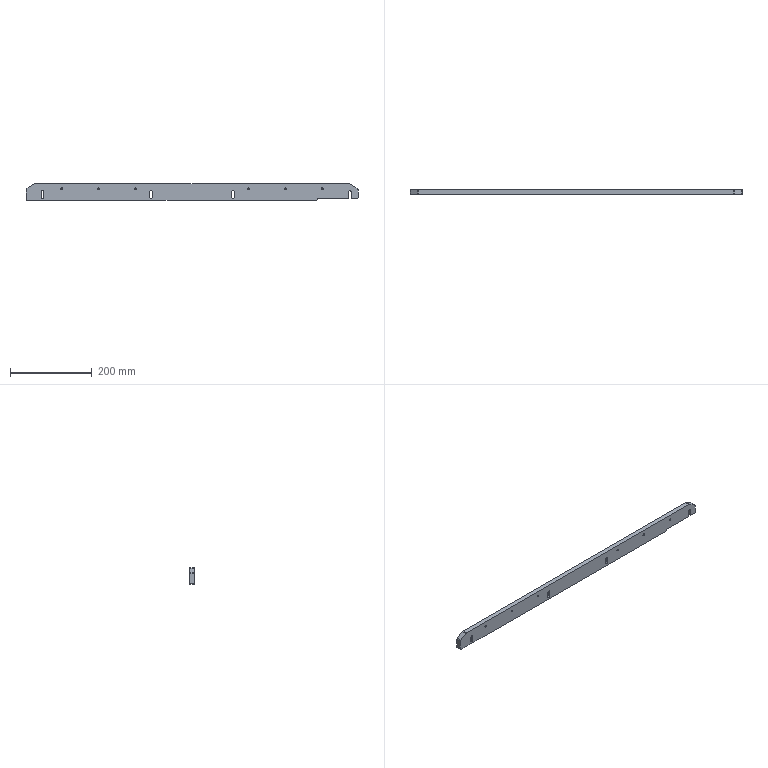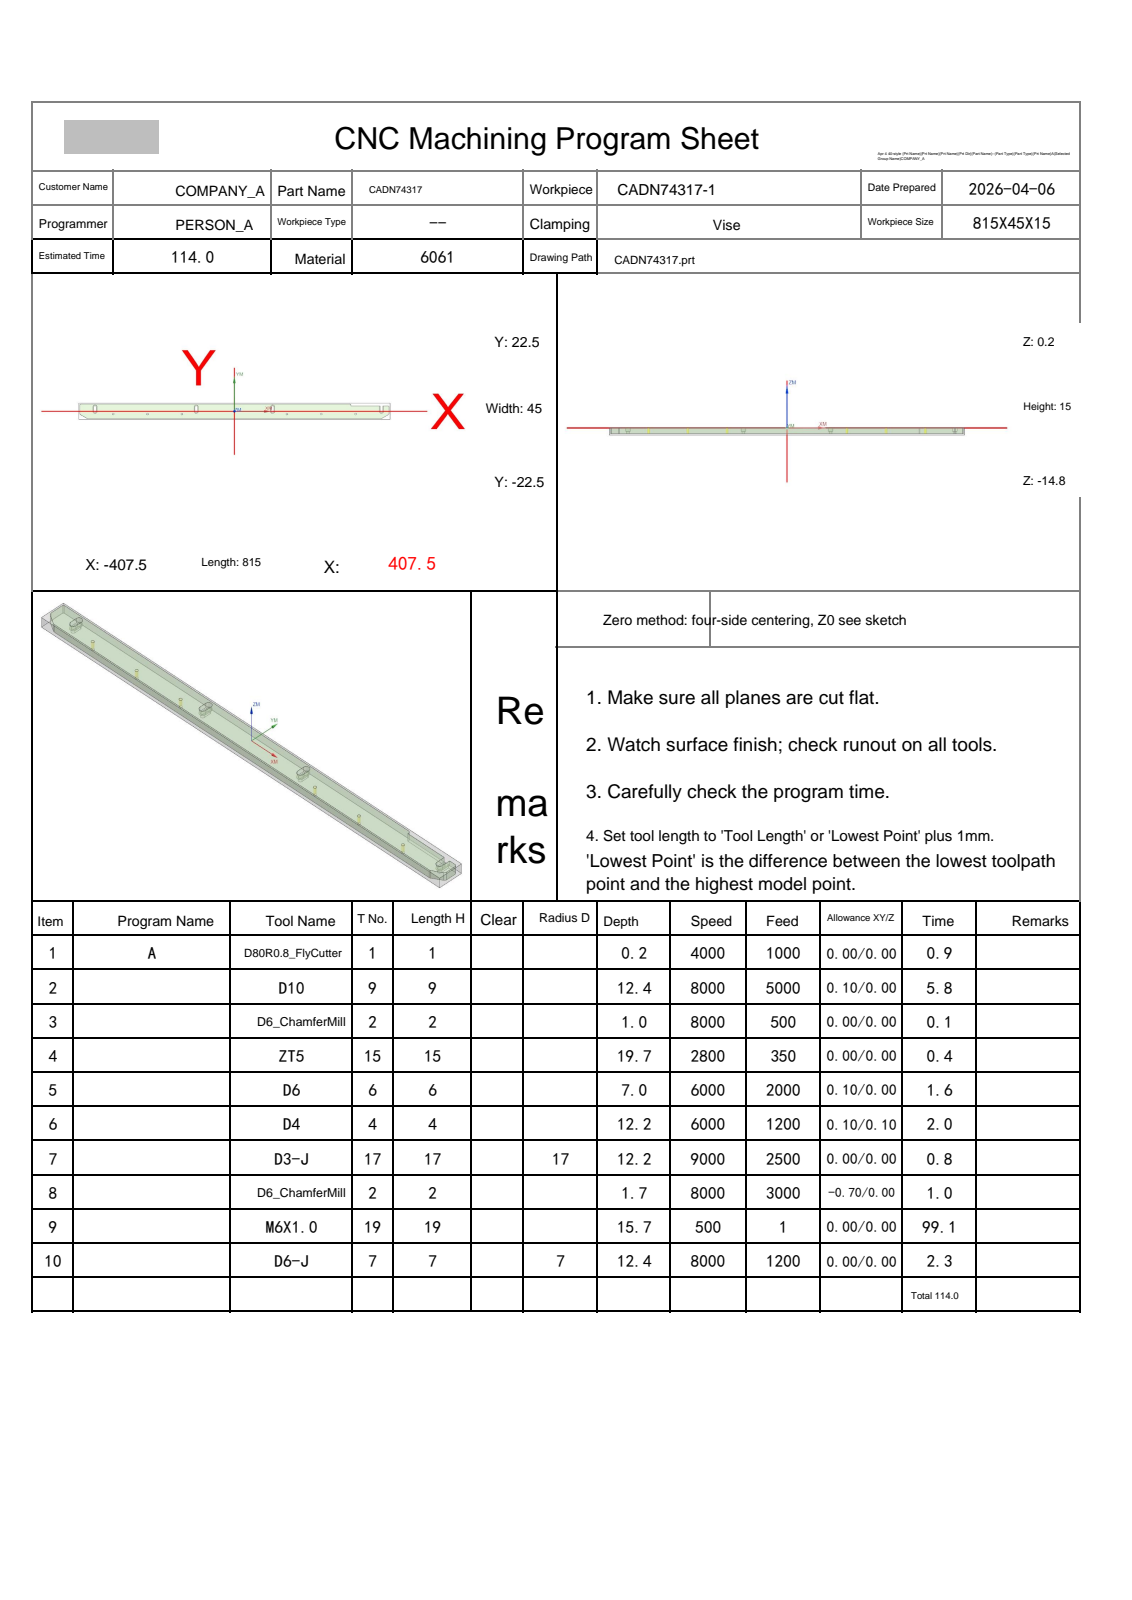NC program | NX | posted by the shop | part box 810 x 12 x 40 mm
Lines 1439 to 3610 of 3610, first 1654 of 2172 lines:
N7 T17 M06
(D3-J  D=3. R=0. H=17 ce=0.00 di=0.00)
G00 G90 G54 X-366.55 Y6.2 M03 S6000
G43 H17 Z20.
M08
Z-8.9
G01 Z-9.4 F800.
G41 D17
X-366.6
G03 X-366.8 Y6. I0.0 J-.2
G01 Y0.0
G03 X-365. Y-1.8 I1.8 J0.0
X-363.2 Y0.0 I0.0 J1.8
G01 Y12.
G03 X-365. Y13.8 I-1.8 J0.0
X-366.8 Y12. I0.0 J-1.8
G01 Y6.
Y5.5
G03 X-366.6 Y5.3 I.2 J0.0
G01 G40 X-366.55
Z-8.9
G00 Z-5.8
Y6.2
Z-11.5
G01 Z-12.
G41 D17
X-366.6
G03 X-366.8 Y6. I0.0 J-.2
G01 Y0.0
G03 X-365. Y-1.8 I1.8 J0.0
X-363.2 Y0.0 I0.0 J1.8
G01 Y12.
G03 X-365. Y13.8 I-1.8 J0.0
X-366.8 Y12. I0.0 J-1.8
G01 Y6.
Y5.5
G03 X-366.6 Y5.3 I.2 J0.0
G01 G40 X-366.55
Z-11.5
G00 Z20.
X-101.55 Y6.2
Z-8.9
G01 Z-9.4
G41 D17
X-101.6
G03 X-101.8 Y6. I0.0 J-.2
G01 Y0.0
G03 X-100. Y-1.8 I1.8 J0.0
X-98.2 Y0.0 I0.0 J1.8
G01 Y12.
G03 X-100. Y13.8 I-1.8 J0.0
X-101.8 Y12. I0.0 J-1.8
G01 Y6.
Y5.5
G03 X-101.6 Y5.3 I.2 J0.0
G01 G40 X-101.55
Z-8.9
G00 Z-5.8
Y6.2
Z-11.5
G01 Z-12.
G41 D17
X-101.6
G03 X-101.8 Y6. I0.0 J-.2
G01 Y0.0
G03 X-100. Y-1.8 I1.8 J0.0
X-98.2 Y0.0 I0.0 J1.8
G01 Y12.
G03 X-100. Y13.8 I-1.8 J0.0
X-101.8 Y12. I0.0 J-1.8
G01 Y6.
Y5.5
G03 X-101.6 Y5.3 I.2 J0.0
G01 G40 X-101.55
Z-11.5
G00 Z20.
X98.45 Y6.2
Z-8.9
G01 Z-9.4
G41 D17
X98.4
G03 X98.2 Y6. I0.0 J-.2
G01 Y0.0
G03 X100. Y-1.8 I1.8 J0.0
X101.8 Y0.0 I0.0 J1.8
G01 Y12.
G03 X100. Y13.8 I-1.8 J0.0
X98.2 Y12. I0.0 J-1.8
G01 Y6.
Y5.5
G03 X98.4 Y5.3 I.2 J0.0
G01 G40 X98.45
Z-8.9
G00 Z-5.8
Y6.2
Z-11.5
G01 Z-12.
G41 D17
X98.4
G03 X98.2 Y6. I0.0 J-.2
G01 Y0.0
G03 X100. Y-1.8 I1.8 J0.0
X101.8 Y0.0 I0.0 J1.8
G01 Y12.
G03 X100. Y13.8 I-1.8 J0.0
X98.2 Y12. I0.0 J-1.8
G01 Y6.
Y5.5
G03 X98.4 Y5.3 I.2 J0.0
G01 G40 X98.45
Z-11.5
G00 Z20.
G00 G90 X306.441 Y19.378 M03 S9000
Z20.
Z.151
G01 X306.438 Y19.374 Z.087 F2000.
X306.427 Y19.364 Z.029
X306.41 Y19.347 Z-.024
X306.389 Y19.324 Z-.071
X306.365 Y19.297 Z-.113
X306.338 Y19.266 Z-.149
X306.311 Y19.23 Z-.181
X306.284 Y19.192 Z-.209
X306.259 Y19.152 Z-.232
X306.236 Y19.109 Z-.251
X306.218 Y19.066 Z-.267
X306.205 Y19.023 Z-.279
X306.198 Y18.98 Z-.288
X306.2 Y18.937 Z-.294
X306.21 Y18.897 Z-.298
X306.23 Y18.859 Z-.299
G02 X306.5 Y18. I-1.23 J-.859 F2500.
G01 Y16.5
X309.708
X309.736 Y16.513 Z-.3
X309.741 Y16.549 Z-.302
X309.723 Y16.606 Z-.306
X309.685 Y16.681 Z-.312
X309.628 Y16.772 Z-.319
X309.555 Y16.876 Z-.327
X309.467 Y16.99 Z-.336
X309.307 Y17.178 Z-.352
X309.191 Y17.305 Z-.363
X309.004 Y17.495 Z-.38
X308.702 Y17.767 Z-.406
X308.379 Y18.02 Z-.434
X308.039 Y18.249 Z-.462
X307.689 Y18.451 Z-.49
X307.333 Y18.621 Z-.517
X307.155 Y18.693 Z-.529
X306.982 Y18.756 Z-.542
X306.816 Y18.808 Z-.553
X306.663 Y18.85 Z-.564
X306.526 Y18.882 Z-.573
X306.41 Y18.902 Z-.582
X306.318 Y18.91 Z-.588
X306.255 Y18.906 Z-.593
X306.224 Y18.889 Z-.596
X306.23 Y18.859 Z-.598
G02 X306.5 Y18. I-1.23 J-.859
G01 Y16.5
X309.708
X309.736 Y16.513
X309.741 Y16.549 Z-.601
X309.723 Y16.606 Z-.605
X309.685 Y16.681 Z-.611
X309.628 Y16.772 Z-.618
X309.555 Y16.876 Z-.626
X309.467 Y16.99 Z-.635
X309.307 Y17.178 Z-.65
X309.191 Y17.305 Z-.661
X309.004 Y17.495 Z-.678
X308.702 Y17.767 Z-.705
X308.379 Y18.02 Z-.733
X308.039 Y18.249 Z-.761
X307.689 Y18.451 Z-.789
X307.333 Y18.621 Z-.815
X307.155 Y18.693 Z-.828
X306.982 Y18.756 Z-.84
X306.816 Y18.808 Z-.852
X306.663 Y18.85 Z-.863
X306.526 Y18.882 Z-.872
X306.41 Y18.902 Z-.88
X306.318 Y18.91 Z-.887
X306.255 Y18.906 Z-.892
X306.224 Y18.889 Z-.895
X306.23 Y18.859 Z-.896
G02 X306.5 Y18. I-1.23 J-.859
G01 Y16.5
X309.708
X309.736 Y16.513 Z-.897
X309.741 Y16.549 Z-.9
X309.723 Y16.606 Z-.904
X309.685 Y16.681 Z-.91
X309.628 Y16.772 Z-.916
X309.555 Y16.876 Z-.925
X309.467 Y16.99 Z-.934
X309.307 Y17.178 Z-.949
X309.191 Y17.305 Z-.96
X309.004 Y17.495 Z-.977
X308.702 Y17.767 Z-1.004
X308.379 Y18.02 Z-1.032
X308.039 Y18.249 Z-1.06
X307.689 Y18.451 Z-1.087
X307.333 Y18.621 Z-1.114
X307.155 Y18.693 Z-1.127
X306.982 Y18.756 Z-1.139
X306.816 Y18.808 Z-1.151
X306.663 Y18.85 Z-1.161
X306.526 Y18.882 Z-1.171
X306.41 Y18.902 Z-1.179
X306.318 Y18.91 Z-1.186
X306.255 Y18.906 Z-1.191
X306.224 Y18.889 Z-1.194
X306.23 Y18.859 Z-1.195
G02 X306.5 Y18. I-1.23 J-.859
G01 Y16.5
X309.708
X309.736 Y16.513 Z-1.196
X309.741 Y16.549 Z-1.199
X309.723 Y16.606 Z-1.203
X309.685 Y16.681 Z-1.208
X309.628 Y16.772 Z-1.215
X309.555 Y16.876 Z-1.223
X309.467 Y16.99 Z-1.232
X309.307 Y17.178 Z-1.248
X309.191 Y17.305 Z-1.259
X309.004 Y17.495 Z-1.276
X308.702 Y17.767 Z-1.303
X308.379 Y18.02 Z-1.33
X308.039 Y18.249 Z-1.358
X307.689 Y18.451 Z-1.386
X307.333 Y18.621 Z-1.413
X307.155 Y18.693 Z-1.426
X306.982 Y18.756 Z-1.438
X306.816 Y18.808 Z-1.45
X306.663 Y18.85 Z-1.46
X306.526 Y18.882 Z-1.47
X306.41 Y18.902 Z-1.478
X306.318 Y18.91 Z-1.485
X306.255 Y18.906 Z-1.49
X306.224 Y18.889 Z-1.493
X306.23 Y18.859 Z-1.494
G02 X306.5 Y18. I-1.23 J-.859
G01 Y16.5
X309.708
X309.736 Y16.513 Z-1.495
X309.741 Y16.549 Z-1.497
X309.723 Y16.606 Z-1.501
X309.685 Y16.681 Z-1.507
X309.628 Y16.772 Z-1.514
X309.555 Y16.876 Z-1.522
X309.467 Y16.99 Z-1.531
X309.307 Y17.178 Z-1.547
X309.191 Y17.305 Z-1.558
X309.004 Y17.495 Z-1.575
X308.702 Y17.767 Z-1.601
X308.379 Y18.02 Z-1.629
X308.039 Y18.249 Z-1.657
X307.689 Y18.451 Z-1.685
X307.333 Y18.621 Z-1.712
X307.155 Y18.693 Z-1.724
X306.982 Y18.756 Z-1.737
X306.816 Y18.808 Z-1.748
X306.663 Y18.85 Z-1.759
X306.526 Y18.882 Z-1.768
X306.41 Y18.902 Z-1.777
X306.318 Y18.91 Z-1.783
X306.255 Y18.906 Z-1.788
X306.224 Y18.889 Z-1.791
X306.23 Y18.859 Z-1.793
G02 X306.5 Y18. I-1.23 J-.859
G01 Y16.5
X309.708
X309.736 Y16.513
X309.741 Y16.549 Z-1.796
X309.723 Y16.606 Z-1.8
X309.685 Y16.681 Z-1.806
X309.628 Y16.772 Z-1.813
X309.555 Y16.876 Z-1.821
X309.467 Y16.99 Z-1.83
X309.307 Y17.178 Z-1.845
X309.191 Y17.305 Z-1.856
X309.004 Y17.495 Z-1.873
X308.702 Y17.767 Z-1.9
X308.379 Y18.02 Z-1.928
X308.039 Y18.249 Z-1.956
X307.689 Y18.451 Z-1.984
X307.333 Y18.621 Z-2.01
X307.155 Y18.693 Z-2.023
X306.982 Y18.756 Z-2.035
X306.816 Y18.808 Z-2.047
X306.663 Y18.85 Z-2.058
X306.526 Y18.882 Z-2.067
X306.41 Y18.902 Z-2.075
X306.318 Y18.91 Z-2.082
X306.255 Y18.906 Z-2.087
X306.224 Y18.889 Z-2.09
X306.23 Y18.859 Z-2.091
G02 X306.5 Y18. I-1.23 J-.859
G01 Y16.5
X309.708
X309.736 Y16.513 Z-2.092
X309.741 Y16.549 Z-2.095
X309.723 Y16.606 Z-2.099
X309.685 Y16.681 Z-2.105
X309.628 Y16.772 Z-2.111
X309.555 Y16.876 Z-2.12
X309.467 Y16.99 Z-2.129
X309.307 Y17.178 Z-2.144
X309.191 Y17.305 Z-2.155
X309.004 Y17.495 Z-2.172
X308.702 Y17.767 Z-2.199
X308.379 Y18.02 Z-2.227
X308.039 Y18.249 Z-2.255
X307.689 Y18.451 Z-2.282
X307.333 Y18.621 Z-2.309
X307.155 Y18.693 Z-2.322
X306.982 Y18.756 Z-2.334
X306.816 Y18.808 Z-2.346
X306.663 Y18.85 Z-2.356
X306.526 Y18.882 Z-2.366
X306.41 Y18.902 Z-2.374
X306.318 Y18.91 Z-2.381
X306.255 Y18.906 Z-2.386
X306.224 Y18.889 Z-2.389
X306.23 Y18.859 Z-2.39
G02 X306.5 Y18. I-1.23 J-.859
G01 Y16.5
X309.708
X309.736 Y16.513 Z-2.391
X309.741 Y16.549 Z-2.394
X309.723 Y16.606 Z-2.398
X309.685 Y16.681 Z-2.403
X309.628 Y16.772 Z-2.41
X309.555 Y16.876 Z-2.418
X309.467 Y16.99 Z-2.427
X309.307 Y17.178 Z-2.443
X309.191 Y17.305 Z-2.454
X309.004 Y17.495 Z-2.471
X308.702 Y17.767 Z-2.498
X308.379 Y18.02 Z-2.525
X308.039 Y18.249 Z-2.553
X307.689 Y18.451 Z-2.581
X307.333 Y18.621 Z-2.608
X307.155 Y18.693 Z-2.621
X306.982 Y18.756 Z-2.633
X306.816 Y18.808 Z-2.645
X306.663 Y18.85 Z-2.655
X306.526 Y18.882 Z-2.665
X306.41 Y18.902 Z-2.673
X306.318 Y18.91 Z-2.68
X306.255 Y18.906 Z-2.685
X306.224 Y18.889 Z-2.688
X306.23 Y18.859 Z-2.689
G02 X306.5 Y18. I-1.23 J-.859
G01 Y16.5
X309.708
X309.736 Y16.513 Z-2.69
X309.741 Y16.549 Z-2.692
X309.723 Y16.606 Z-2.696
X309.685 Y16.681 Z-2.702
X309.628 Y16.772 Z-2.709
X309.555 Y16.876 Z-2.717
X309.467 Y16.99 Z-2.726
X309.307 Y17.178 Z-2.742
X309.191 Y17.305 Z-2.753
X309.004 Y17.495 Z-2.77
X308.702 Y17.767 Z-2.796
X308.379 Y18.02 Z-2.824
X308.039 Y18.249 Z-2.852
X307.689 Y18.451 Z-2.88
X307.333 Y18.621 Z-2.907
X307.155 Y18.693 Z-2.919
X306.982 Y18.756 Z-2.932
X306.816 Y18.808 Z-2.943
X306.663 Y18.85 Z-2.954
X306.526 Y18.882 Z-2.963
X306.41 Y18.902 Z-2.972
X306.318 Y18.91 Z-2.978
X306.255 Y18.906 Z-2.983
X306.224 Y18.889 Z-2.986
X306.23 Y18.859 Z-2.988
G02 X306.5 Y18. I-1.23 J-.859
G01 Y16.5
X309.708
X309.736 Y16.513
X309.741 Y16.549 Z-2.991
X309.723 Y16.606 Z-2.995
X309.685 Y16.681 Z-3.001
X309.628 Y16.772 Z-3.008
X309.555 Y16.876 Z-3.016
X309.467 Y16.99 Z-3.025
X309.307 Y17.178 Z-3.04
X309.191 Y17.305 Z-3.051
X309.004 Y17.495 Z-3.068
X308.702 Y17.767 Z-3.095
X308.379 Y18.02 Z-3.123
X308.039 Y18.249 Z-3.151
X307.689 Y18.451 Z-3.179
X307.333 Y18.621 Z-3.205
X307.155 Y18.693 Z-3.218
X306.982 Y18.756 Z-3.23
X306.816 Y18.808 Z-3.242
X306.663 Y18.85 Z-3.253
X306.526 Y18.882 Z-3.262
X306.41 Y18.902 Z-3.27
X306.318 Y18.91 Z-3.277
X306.255 Y18.906 Z-3.282
X306.224 Y18.889 Z-3.285
X306.23 Y18.859 Z-3.286
G02 X306.5 Y18. I-1.23 J-.859
G01 Y16.5
X309.708
X309.736 Y16.513 Z-3.287
X309.741 Y16.549 Z-3.29
X309.723 Y16.606 Z-3.294
X309.685 Y16.681 Z-3.3
X309.628 Y16.772 Z-3.306
X309.555 Y16.876 Z-3.315
X309.467 Y16.99 Z-3.324
X309.307 Y17.178 Z-3.339
X309.191 Y17.305 Z-3.35
X309.004 Y17.495 Z-3.367
X308.702 Y17.767 Z-3.394
X308.379 Y18.02 Z-3.422
X308.039 Y18.249 Z-3.45
X307.689 Y18.451 Z-3.477
X307.333 Y18.621 Z-3.504
X307.155 Y18.693 Z-3.517
X306.982 Y18.756 Z-3.529
X306.816 Y18.808 Z-3.541
X306.663 Y18.85 Z-3.551
X306.526 Y18.882 Z-3.561
X306.41 Y18.902 Z-3.569
X306.318 Y18.91 Z-3.576
X306.255 Y18.906 Z-3.581
X306.224 Y18.889 Z-3.584
X306.23 Y18.859 Z-3.585
G02 X306.5 Y18. I-1.23 J-.859
G01 Y16.5
X309.708
X309.736 Y16.513 Z-3.586
X309.741 Y16.549 Z-3.589
X309.723 Y16.606 Z-3.593
X309.685 Y16.681 Z-3.598
X309.628 Y16.772 Z-3.605
X309.555 Y16.876 Z-3.613
X309.467 Y16.99 Z-3.622
X309.307 Y17.178 Z-3.638
X309.191 Y17.305 Z-3.649
X309.004 Y17.495 Z-3.666
X308.702 Y17.767 Z-3.693
X308.379 Y18.02 Z-3.72
X308.039 Y18.249 Z-3.748
X307.689 Y18.451 Z-3.776
X307.333 Y18.621 Z-3.803
X307.155 Y18.693 Z-3.816
X306.982 Y18.756 Z-3.828
X306.816 Y18.808 Z-3.84
X306.663 Y18.85 Z-3.85
X306.526 Y18.882 Z-3.86
X306.41 Y18.902 Z-3.868
X306.318 Y18.91 Z-3.875
X306.255 Y18.906 Z-3.88
X306.224 Y18.889 Z-3.883
X306.23 Y18.859 Z-3.884
G02 X306.5 Y18. I-1.23 J-.859
G01 Y16.5
X309.708
X309.736 Y16.513 Z-3.885
X309.741 Y16.549 Z-3.887
X309.723 Y16.606 Z-3.891
X309.685 Y16.681 Z-3.897
X309.628 Y16.772 Z-3.904
X309.555 Y16.876 Z-3.912
X309.467 Y16.99 Z-3.921
X309.307 Y17.178 Z-3.937
X309.191 Y17.305 Z-3.948
X309.004 Y17.495 Z-3.965
X308.702 Y17.767 Z-3.991
X308.379 Y18.02 Z-4.019
X308.039 Y18.249 Z-4.047
X307.689 Y18.451 Z-4.075
X307.333 Y18.621 Z-4.102
X307.155 Y18.693 Z-4.114
X306.982 Y18.756 Z-4.127
X306.816 Y18.808 Z-4.138
X306.663 Y18.85 Z-4.149
X306.526 Y18.882 Z-4.158
X306.41 Y18.902 Z-4.167
X306.318 Y18.91 Z-4.173
X306.255 Y18.906 Z-4.178
X306.224 Y18.889 Z-4.181
X306.23 Y18.859 Z-4.183
G02 X306.5 Y18. I-1.23 J-.859
G01 Y16.5
X309.708
X309.736 Y16.513
X309.741 Y16.549 Z-4.186
X309.723 Y16.606 Z-4.19
X309.685 Y16.681 Z-4.196
X309.628 Y16.772 Z-4.203
X309.555 Y16.876 Z-4.211
X309.467 Y16.99 Z-4.22
X309.307 Y17.178 Z-4.235
X309.191 Y17.305 Z-4.246
X309.004 Y17.495 Z-4.263
X308.702 Y17.767 Z-4.29
X308.379 Y18.02 Z-4.318
X308.039 Y18.249 Z-4.346
X307.689 Y18.451 Z-4.374
X307.333 Y18.621 Z-4.4
X307.155 Y18.693 Z-4.413
X306.982 Y18.756 Z-4.425
X306.816 Y18.808 Z-4.437
X306.663 Y18.85 Z-4.448
X306.526 Y18.882 Z-4.457
X306.41 Y18.902 Z-4.465
X306.318 Y18.91 Z-4.472
X306.255 Y18.906 Z-4.477
X306.224 Y18.889 Z-4.48
X306.23 Y18.859 Z-4.481
G02 X306.5 Y18. I-1.23 J-.859
G01 Y16.5
X309.708
X309.736 Y16.513 Z-4.482
X309.741 Y16.549 Z-4.485
X309.723 Y16.606 Z-4.489
X309.685 Y16.681 Z-4.495
X309.628 Y16.772 Z-4.501
X309.555 Y16.876 Z-4.51
X309.467 Y16.99 Z-4.519
X309.307 Y17.178 Z-4.534
X309.191 Y17.305 Z-4.545
X309.004 Y17.495 Z-4.562
X308.702 Y17.767 Z-4.589
X308.379 Y18.02 Z-4.617
X308.039 Y18.249 Z-4.645
X307.689 Y18.451 Z-4.672
X307.333 Y18.621 Z-4.699
X307.155 Y18.693 Z-4.712
X306.982 Y18.756 Z-4.724
X306.816 Y18.808 Z-4.736
X306.663 Y18.85 Z-4.746
X306.526 Y18.882 Z-4.756
X306.41 Y18.902 Z-4.764
X306.318 Y18.91 Z-4.771
X306.255 Y18.906 Z-4.776
X306.224 Y18.889 Z-4.779
X306.23 Y18.859 Z-4.78
G02 X306.5 Y18. I-1.23 J-.859
G01 Y16.5
X309.708
X309.736 Y16.513 Z-4.781
X309.741 Y16.549 Z-4.784
X309.723 Y16.606 Z-4.788
X309.685 Y16.681 Z-4.793
X309.628 Y16.772 Z-4.8
X309.555 Y16.876 Z-4.808
X309.467 Y16.99 Z-4.817
X309.307 Y17.178 Z-4.833
X309.191 Y17.305 Z-4.844
X309.004 Y17.495 Z-4.861
X308.702 Y17.767 Z-4.888
X308.379 Y18.02 Z-4.915
X308.039 Y18.249 Z-4.943
X307.689 Y18.451 Z-4.971
X307.333 Y18.621 Z-4.998
X307.155 Y18.693 Z-5.011
X306.982 Y18.756 Z-5.023
X306.816 Y18.808 Z-5.035
X306.663 Y18.85 Z-5.045
X306.526 Y18.882 Z-5.055
X306.41 Y18.902 Z-5.063
X306.318 Y18.91 Z-5.07
X306.255 Y18.906 Z-5.075
X306.224 Y18.889 Z-5.078
X306.23 Y18.859 Z-5.079
G02 X306.5 Y18. I-1.23 J-.859
G01 Y16.5
X309.708
X309.736 Y16.513 Z-5.08
X309.741 Y16.549 Z-5.082
X309.723 Y16.606 Z-5.086
X309.685 Y16.681 Z-5.092
X309.628 Y16.772 Z-5.099
X309.555 Y16.876 Z-5.107
X309.467 Y16.99 Z-5.116
X309.307 Y17.178 Z-5.132
X309.191 Y17.305 Z-5.143
X309.004 Y17.495 Z-5.16
X308.702 Y17.767 Z-5.186
X308.379 Y18.02 Z-5.214
X308.039 Y18.249 Z-5.242
X307.689 Y18.451 Z-5.27
X307.333 Y18.621 Z-5.297
X307.155 Y18.693 Z-5.309
X306.982 Y18.756 Z-5.322
X306.816 Y18.808 Z-5.333
X306.663 Y18.85 Z-5.344
X306.526 Y18.882 Z-5.353
X306.41 Y18.902 Z-5.362
X306.318 Y18.91 Z-5.368
X306.255 Y18.906 Z-5.373
X306.224 Y18.889 Z-5.376
X306.23 Y18.859 Z-5.378
G02 X306.5 Y18. I-1.23 J-.859
G01 Y16.5
X309.708
X309.736 Y16.513
X309.741 Y16.549 Z-5.381
X309.723 Y16.606 Z-5.385
X309.685 Y16.681 Z-5.391
X309.628 Y16.772 Z-5.398
X309.555 Y16.876 Z-5.406
X309.467 Y16.99 Z-5.415
X309.307 Y17.178 Z-5.43
X309.191 Y17.305 Z-5.441
X309.004 Y17.495 Z-5.458
X308.702 Y17.767 Z-5.485
X308.379 Y18.02 Z-5.513
X308.039 Y18.249 Z-5.541
X307.689 Y18.451 Z-5.569
X307.333 Y18.621 Z-5.595
X307.155 Y18.693 Z-5.608
X306.982 Y18.756 Z-5.62
X306.816 Y18.808 Z-5.632
X306.663 Y18.85 Z-5.643
X306.526 Y18.882 Z-5.652
X306.41 Y18.902 Z-5.66
X306.318 Y18.91 Z-5.667
X306.255 Y18.906 Z-5.672
X306.224 Y18.889 Z-5.675
X306.23 Y18.859 Z-5.676
G02 X306.5 Y18. I-1.23 J-.859
G01 Y16.5
X309.708
X309.736 Y16.513 Z-5.677
X309.741 Y16.549 Z-5.68
X309.723 Y16.606 Z-5.684
X309.685 Y16.681 Z-5.69
X309.628 Y16.772 Z-5.696
X309.555 Y16.876 Z-5.705
X309.467 Y16.99 Z-5.714
X309.307 Y17.178 Z-5.729
X309.191 Y17.305 Z-5.74
X309.004 Y17.495 Z-5.757
X308.702 Y17.767 Z-5.784
X308.379 Y18.02 Z-5.812
X308.039 Y18.249 Z-5.84
X307.689 Y18.451 Z-5.867
X307.333 Y18.621 Z-5.894
X307.155 Y18.693 Z-5.907
X306.982 Y18.756 Z-5.919
X306.816 Y18.808 Z-5.931
X306.663 Y18.85 Z-5.941
X306.526 Y18.882 Z-5.951
X306.41 Y18.902 Z-5.959
X306.318 Y18.91 Z-5.966
X306.255 Y18.906 Z-5.971
X306.224 Y18.889 Z-5.974
X306.23 Y18.859 Z-5.975
G02 X306.5 Y18. I-1.23 J-.859
G01 Y16.5
X309.708
X309.736 Y16.513 Z-5.976
X309.741 Y16.549 Z-5.979
X309.723 Y16.606 Z-5.983
X309.685 Y16.681 Z-5.988
X309.628 Y16.772 Z-5.995
X309.555 Y16.876 Z-6.003
X309.467 Y16.99 Z-6.012
X309.307 Y17.178 Z-6.028
X309.191 Y17.305 Z-6.039
X309.004 Y17.495 Z-6.056
X308.702 Y17.767 Z-6.083
X308.379 Y18.02 Z-6.11
X308.039 Y18.249 Z-6.138
X307.689 Y18.451 Z-6.166
X307.333 Y18.621 Z-6.193
X307.155 Y18.693 Z-6.206
X306.982 Y18.756 Z-6.218
X306.816 Y18.808 Z-6.23
X306.663 Y18.85 Z-6.24
X306.526 Y18.882 Z-6.25
X306.41 Y18.902 Z-6.258
X306.318 Y18.91 Z-6.265
X306.255 Y18.906 Z-6.27
X306.224 Y18.889 Z-6.273
X306.23 Y18.859 Z-6.274
G02 X306.5 Y18. I-1.23 J-.859
G01 Y16.5
X309.708
X309.736 Y16.513 Z-6.275
X309.741 Y16.549 Z-6.277
X309.723 Y16.606 Z-6.281
X309.685 Y16.681 Z-6.287
X309.628 Y16.772 Z-6.294
X309.555 Y16.876 Z-6.302
X309.467 Y16.99 Z-6.311
X309.307 Y17.178 Z-6.327
X309.191 Y17.305 Z-6.338
X309.004 Y17.495 Z-6.355
X308.702 Y17.767 Z-6.381
X308.379 Y18.02 Z-6.409
X308.039 Y18.249 Z-6.437
X307.689 Y18.451 Z-6.465
X307.333 Y18.621 Z-6.492
X307.155 Y18.693 Z-6.504
X306.982 Y18.756 Z-6.517
X306.816 Y18.808 Z-6.528
X306.663 Y18.85 Z-6.539
X306.526 Y18.882 Z-6.548
X306.41 Y18.902 Z-6.557
X306.318 Y18.91 Z-6.563
X306.255 Y18.906 Z-6.568
X306.224 Y18.889 Z-6.571
X306.23 Y18.859 Z-6.573
G02 X306.5 Y18. I-1.23 J-.859
G01 Y16.5
X309.708
X309.736 Y16.513
X309.741 Y16.549 Z-6.576
X309.723 Y16.606 Z-6.58
X309.685 Y16.681 Z-6.586
X309.628 Y16.772 Z-6.593
X309.555 Y16.876 Z-6.601
X309.467 Y16.99 Z-6.61
X309.307 Y17.178 Z-6.625
X309.191 Y17.305 Z-6.636
X309.004 Y17.495 Z-6.653
X308.702 Y17.767 Z-6.68
X308.379 Y18.02 Z-6.708
X308.039 Y18.249 Z-6.736
X307.689 Y18.451 Z-6.764
X307.333 Y18.621 Z-6.79
X307.155 Y18.693 Z-6.803
X306.982 Y18.756 Z-6.815
X306.816 Y18.808 Z-6.827
X306.663 Y18.85 Z-6.838
X306.526 Y18.882 Z-6.847
X306.41 Y18.902 Z-6.855
X306.318 Y18.91 Z-6.862
X306.255 Y18.906 Z-6.867
X306.224 Y18.889 Z-6.87
X306.23 Y18.859 Z-6.871
G02 X306.5 Y18. I-1.23 J-.859
G01 Y16.5
X309.708
X309.736 Y16.513 Z-6.872
X309.741 Y16.549 Z-6.875
X309.723 Y16.606 Z-6.879
X309.685 Y16.681 Z-6.885
X309.628 Y16.772 Z-6.891
X309.555 Y16.876 Z-6.9
X309.467 Y16.99 Z-6.909
X309.307 Y17.178 Z-6.924
X309.191 Y17.305 Z-6.935
X309.004 Y17.495 Z-6.952
X308.702 Y17.767 Z-6.979
X308.379 Y18.02 Z-7.007
X308.039 Y18.249 Z-7.035
X307.689 Y18.451 Z-7.062
X307.333 Y18.621 Z-7.089
X307.155 Y18.693 Z-7.102
X306.982 Y18.756 Z-7.114
X306.816 Y18.808 Z-7.126
X306.663 Y18.85 Z-7.136
X306.526 Y18.882 Z-7.146
X306.41 Y18.902 Z-7.154
X306.318 Y18.91 Z-7.161
X306.255 Y18.906 Z-7.166
X306.224 Y18.889 Z-7.169
X306.23 Y18.859 Z-7.17
G02 X306.5 Y18. I-1.23 J-.859
G01 Y16.5
X309.708
X309.736 Y16.513 Z-7.171
X309.741 Y16.549 Z-7.174
X309.723 Y16.606 Z-7.178
X309.685 Y16.681 Z-7.183
X309.628 Y16.772 Z-7.19
X309.555 Y16.876 Z-7.198
X309.467 Y16.99 Z-7.207
X309.307 Y17.178 Z-7.223
X309.191 Y17.305 Z-7.234
X309.004 Y17.495 Z-7.251
X308.702 Y17.767 Z-7.278
X308.379 Y18.02 Z-7.305
X308.039 Y18.249 Z-7.333
X307.689 Y18.451 Z-7.361
X307.333 Y18.621 Z-7.388
X307.155 Y18.693 Z-7.401
X306.982 Y18.756 Z-7.413
X306.816 Y18.808 Z-7.425
X306.663 Y18.85 Z-7.435
X306.526 Y18.882 Z-7.445
X306.41 Y18.902 Z-7.453
X306.318 Y18.91 Z-7.46
X306.255 Y18.906 Z-7.465
X306.224 Y18.889 Z-7.468
X306.23 Y18.859 Z-7.469
G02 X306.5 Y18. I-1.23 J-.859
G01 Y16.5
X309.708
X309.736 Y16.513 Z-7.47
X309.741 Y16.549 Z-7.472
X309.723 Y16.606 Z-7.476
X309.685 Y16.681 Z-7.482
X309.628 Y16.772 Z-7.489
X309.555 Y16.876 Z-7.497
X309.467 Y16.99 Z-7.506
X309.307 Y17.178 Z-7.522
X309.191 Y17.305 Z-7.533
X309.004 Y17.495 Z-7.55
X308.702 Y17.767 Z-7.576
X308.379 Y18.02 Z-7.604
X308.039 Y18.249 Z-7.632
X307.689 Y18.451 Z-7.66
X307.333 Y18.621 Z-7.687
X307.155 Y18.693 Z-7.699
X306.982 Y18.756 Z-7.712
X306.816 Y18.808 Z-7.723
X306.663 Y18.85 Z-7.734
X306.526 Y18.882 Z-7.743
X306.41 Y18.902 Z-7.752
X306.318 Y18.91 Z-7.758
X306.255 Y18.906 Z-7.763
X306.224 Y18.889 Z-7.766
X306.23 Y18.859 Z-7.768
G02 X306.5 Y18. I-1.23 J-.859
G01 Y16.5
X309.708
X309.736 Y16.513
X309.741 Y16.549 Z-7.771
X309.723 Y16.606 Z-7.775
X309.685 Y16.681 Z-7.781
X309.628 Y16.772 Z-7.788
X309.555 Y16.876 Z-7.796
X309.467 Y16.99 Z-7.805
X309.307 Y17.178 Z-7.82
X309.191 Y17.305 Z-7.831
X309.004 Y17.495 Z-7.848
X308.702 Y17.767 Z-7.875
X308.379 Y18.02 Z-7.903
X308.039 Y18.249 Z-7.931
X307.689 Y18.451 Z-7.959
X307.333 Y18.621 Z-7.985
X307.155 Y18.693 Z-7.998
X306.982 Y18.756 Z-8.01
X306.816 Y18.808 Z-8.022
X306.663 Y18.85 Z-8.033
X306.526 Y18.882 Z-8.042
X306.41 Y18.902 Z-8.05
X306.318 Y18.91 Z-8.057
X306.255 Y18.906 Z-8.062
X306.224 Y18.889 Z-8.065
X306.23 Y18.859 Z-8.066
G02 X306.5 Y18. I-1.23 J-.859
G01 Y16.5
X309.708
X309.736 Y16.513 Z-8.067
X309.741 Y16.549 Z-8.07
X309.723 Y16.606 Z-8.074
X309.685 Y16.681 Z-8.08
X309.628 Y16.772 Z-8.086
X309.555 Y16.876 Z-8.095
X309.467 Y16.99 Z-8.104
X309.307 Y17.178 Z-8.119
X309.191 Y17.305 Z-8.13
X309.004 Y17.495 Z-8.147
X308.702 Y17.767 Z-8.174
X308.379 Y18.02 Z-8.202
X308.039 Y18.249 Z-8.23
X307.689 Y18.451 Z-8.257
X307.333 Y18.621 Z-8.284
X307.155 Y18.693 Z-8.297
X306.982 Y18.756 Z-8.309
X306.816 Y18.808 Z-8.321
X306.663 Y18.85 Z-8.331
X306.526 Y18.882 Z-8.341
X306.41 Y18.902 Z-8.349
X306.318 Y18.91 Z-8.356
X306.255 Y18.906 Z-8.361
X306.224 Y18.889 Z-8.364
X306.23 Y18.859 Z-8.365
G02 X306.5 Y18. I-1.23 J-.859
G01 Y16.5
X309.708
X309.736 Y16.513 Z-8.366
X309.741 Y16.549 Z-8.369
X309.723 Y16.606 Z-8.373
X309.685 Y16.681 Z-8.378
X309.628 Y16.772 Z-8.385
X309.555 Y16.876 Z-8.393
X309.467 Y16.99 Z-8.402
X309.307 Y17.178 Z-8.418
X309.191 Y17.305 Z-8.429
X309.004 Y17.495 Z-8.446
X308.702 Y17.767 Z-8.473
X308.379 Y18.02 Z-8.5
X308.039 Y18.249 Z-8.528
X307.689 Y18.451 Z-8.556
X307.333 Y18.621 Z-8.583
X307.155 Y18.693 Z-8.596
X306.982 Y18.756 Z-8.608
X306.816 Y18.808 Z-8.62
X306.663 Y18.85 Z-8.63
X306.526 Y18.882 Z-8.64
X306.41 Y18.902 Z-8.648
X306.318 Y18.91 Z-8.655
X306.255 Y18.906 Z-8.66
X306.224 Y18.889 Z-8.663
X306.23 Y18.859 Z-8.664
G02 X306.5 Y18. I-1.23 J-.859
G01 Y16.5
X309.708
X309.736 Y16.513 Z-8.665
X309.741 Y16.549 Z-8.667
X309.723 Y16.606 Z-8.671
X309.685 Y16.681 Z-8.677
X309.628 Y16.772 Z-8.684
X309.555 Y16.876 Z-8.692
X309.467 Y16.99 Z-8.701
X309.307 Y17.178 Z-8.717
X309.191 Y17.305 Z-8.728
X309.004 Y17.495 Z-8.745
X308.702 Y17.767 Z-8.771
X308.379 Y18.02 Z-8.799
X308.039 Y18.249 Z-8.827
X307.689 Y18.451 Z-8.855
X307.333 Y18.621 Z-8.882
X307.155 Y18.693 Z-8.894
X306.982 Y18.756 Z-8.907
X306.816 Y18.808 Z-8.918
X306.663 Y18.85 Z-8.929
X306.526 Y18.882 Z-8.938
X306.41 Y18.902 Z-8.947
X306.318 Y18.91 Z-8.953
X306.255 Y18.906 Z-8.958
X306.224 Y18.889 Z-8.961
X306.23 Y18.859 Z-8.963
G02 X306.5 Y18. I-1.23 J-.859
G01 Y16.5
X309.708
X309.736 Y16.513
X309.741 Y16.549 Z-8.966
X309.723 Y16.606 Z-8.97
X309.685 Y16.681 Z-8.976
X309.628 Y16.772 Z-8.983
X309.555 Y16.876 Z-8.991
X309.467 Y16.99 Z-9.
X309.307 Y17.178 Z-9.015
X309.191 Y17.305 Z-9.026
X309.004 Y17.495 Z-9.043
X308.702 Y17.767 Z-9.07
X308.379 Y18.02 Z-9.098
X308.039 Y18.249 Z-9.126
X307.689 Y18.451 Z-9.154
X307.333 Y18.621 Z-9.18
X307.155 Y18.693 Z-9.193
X306.982 Y18.756 Z-9.205
X306.816 Y18.808 Z-9.217
X306.663 Y18.85 Z-9.228
X306.526 Y18.882 Z-9.237
X306.41 Y18.902 Z-9.245
X306.318 Y18.91 Z-9.252
X306.255 Y18.906 Z-9.257
X306.224 Y18.889 Z-9.26
X306.23 Y18.859 Z-9.261
G02 X306.5 Y18. I-1.23 J-.859
G01 Y16.5
X309.708
X309.736 Y16.513 Z-9.262
X309.741 Y16.549 Z-9.265
X309.723 Y16.606 Z-9.269
X309.685 Y16.681 Z-9.275
X309.628 Y16.772 Z-9.281
X309.555 Y16.876 Z-9.29
X309.467 Y16.99 Z-9.299
X309.307 Y17.178 Z-9.314
X309.191 Y17.305 Z-9.325
X309.004 Y17.495 Z-9.342
X308.702 Y17.767 Z-9.369
X308.379 Y18.02 Z-9.397
X308.039 Y18.249 Z-9.425
X307.689 Y18.451 Z-9.452
X307.333 Y18.621 Z-9.479
X307.155 Y18.693 Z-9.492
X306.982 Y18.756 Z-9.504
X306.816 Y18.808 Z-9.516
X306.663 Y18.85 Z-9.526
X306.526 Y18.882 Z-9.536
X306.41 Y18.902 Z-9.544
X306.318 Y18.91 Z-9.551
X306.255 Y18.906 Z-9.556
X306.224 Y18.889 Z-9.559
X306.23 Y18.859 Z-9.56
G02 X306.5 Y18. I-1.23 J-.859
G01 Y16.5
X309.708
X309.736 Y16.513 Z-9.561
X309.741 Y16.549 Z-9.564
X309.723 Y16.606 Z-9.568
X309.685 Y16.681 Z-9.573
X309.628 Y16.772 Z-9.58
X309.555 Y16.876 Z-9.588
X309.467 Y16.99 Z-9.597
X309.307 Y17.178 Z-9.613
X309.191 Y17.305 Z-9.624
X309.004 Y17.495 Z-9.641
X308.702 Y17.767 Z-9.668
X308.379 Y18.02 Z-9.695
X308.039 Y18.249 Z-9.723
X307.689 Y18.451 Z-9.751
X307.333 Y18.621 Z-9.778
X307.155 Y18.693 Z-9.791
X306.982 Y18.756 Z-9.803
X306.816 Y18.808 Z-9.815
X306.663 Y18.85 Z-9.825
X306.526 Y18.882 Z-9.835
X306.41 Y18.902 Z-9.843
X306.318 Y18.91 Z-9.85
X306.255 Y18.906 Z-9.855
X306.224 Y18.889 Z-9.858
X306.23 Y18.859 Z-9.859
G02 X306.5 Y18. I-1.23 J-.859
G01 Y16.5
X309.708
X309.736 Y16.513 Z-9.86
X309.741 Y16.549 Z-9.862
X309.723 Y16.606 Z-9.866
X309.685 Y16.681 Z-9.872
X309.628 Y16.772 Z-9.879
X309.555 Y16.876 Z-9.887
X309.467 Y16.99 Z-9.896
X309.307 Y17.178 Z-9.912
X309.191 Y17.305 Z-9.923
X309.004 Y17.495 Z-9.94
X308.702 Y17.767 Z-9.966
X308.379 Y18.02 Z-9.994
X308.039 Y18.249 Z-10.022
X307.689 Y18.451 Z-10.05
X307.333 Y18.621 Z-10.077
X307.155 Y18.693 Z-10.089
X306.982 Y18.756 Z-10.102
X306.816 Y18.808 Z-10.113
X306.663 Y18.85 Z-10.124
X306.526 Y18.882 Z-10.133
X306.41 Y18.902 Z-10.142
X306.318 Y18.91 Z-10.148
X306.255 Y18.906 Z-10.153
X306.224 Y18.889 Z-10.156
X306.23 Y18.859 Z-10.158
G02 X306.5 Y18. I-1.23 J-.859
G01 Y16.5
X309.708
X309.736 Y16.513
X309.741 Y16.549 Z-10.161
X309.723 Y16.606 Z-10.165
X309.685 Y16.681 Z-10.171
X309.628 Y16.772 Z-10.178
X309.555 Y16.876 Z-10.186
X309.467 Y16.99 Z-10.195
X309.307 Y17.178 Z-10.21
X309.191 Y17.305 Z-10.221
X309.004 Y17.495 Z-10.238
X308.702 Y17.767 Z-10.265
X308.379 Y18.02 Z-10.293
X308.039 Y18.249 Z-10.321
X307.689 Y18.451 Z-10.349
X307.333 Y18.621 Z-10.375
X307.155 Y18.693 Z-10.388
X306.982 Y18.756 Z-10.4
X306.816 Y18.808 Z-10.412
X306.663 Y18.85 Z-10.423
X306.526 Y18.882 Z-10.432
X306.41 Y18.902 Z-10.44
X306.318 Y18.91 Z-10.447
X306.255 Y18.906 Z-10.452
X306.224 Y18.889 Z-10.455
X306.23 Y18.859 Z-10.456
G02 X306.5 Y18. I-1.23 J-.859
G01 Y16.5
X309.708
X309.736 Y16.513 Z-10.457
X309.741 Y16.549 Z-10.46
X309.723 Y16.606 Z-10.464
X309.685 Y16.681 Z-10.47
X309.628 Y16.772 Z-10.476
X309.555 Y16.876 Z-10.485
X309.467 Y16.99 Z-10.494
X309.307 Y17.178 Z-10.509
X309.191 Y17.305 Z-10.52
X309.004 Y17.495 Z-10.537
X308.702 Y17.767 Z-10.564
X308.379 Y18.02 Z-10.592
X308.039 Y18.249 Z-10.62
X307.689 Y18.451 Z-10.647
X307.333 Y18.621 Z-10.674
X307.155 Y18.693 Z-10.687
X306.982 Y18.756 Z-10.699
X306.816 Y18.808 Z-10.711
X306.663 Y18.85 Z-10.721
X306.526 Y18.882 Z-10.731
X306.41 Y18.902 Z-10.739
X306.318 Y18.91 Z-10.746
X306.255 Y18.906 Z-10.751
X306.224 Y18.889 Z-10.754
X306.23 Y18.859 Z-10.755
G02 X306.5 Y18. I-1.23 J-.859
G01 Y16.5
X309.708
X309.736 Y16.513 Z-10.756
X309.741 Y16.549 Z-10.759
X309.723 Y16.606 Z-10.763
X309.685 Y16.681 Z-10.768
X309.628 Y16.772 Z-10.775
X309.555 Y16.876 Z-10.783
X309.467 Y16.99 Z-10.792
X309.307 Y17.178 Z-10.808
X309.191 Y17.305 Z-10.819
X309.004 Y17.495 Z-10.836
X308.702 Y17.767 Z-10.863
X308.379 Y18.02 Z-10.89
X308.039 Y18.249 Z-10.918
X307.689 Y18.451 Z-10.946
X307.333 Y18.621 Z-10.973
X307.155 Y18.693 Z-10.986
X306.982 Y18.756 Z-10.998
X306.816 Y18.808 Z-11.01
X306.663 Y18.85 Z-11.02
X306.526 Y18.882 Z-11.03
X306.41 Y18.902 Z-11.038
X306.318 Y18.91 Z-11.045
X306.255 Y18.906 Z-11.05
X306.224 Y18.889 Z-11.053
X306.23 Y18.859 Z-11.054
G02 X306.5 Y18. I-1.23 J-.859
G01 Y16.5
X309.708
X309.736 Y16.513 Z-11.055
X309.741 Y16.549 Z-11.057
X309.723 Y16.606 Z-11.061
X309.685 Y16.681 Z-11.067
X309.628 Y16.772 Z-11.074
X309.555 Y16.876 Z-11.082
X309.467 Y16.99 Z-11.091
X309.307 Y17.178 Z-11.107
X309.191 Y17.305 Z-11.118
X309.004 Y17.495 Z-11.135
X308.702 Y17.767 Z-11.161
X308.379 Y18.02 Z-11.189
X308.039 Y18.249 Z-11.217
X307.689 Y18.451 Z-11.245
X307.333 Y18.621 Z-11.272
X307.155 Y18.693 Z-11.284
X306.982 Y18.756 Z-11.297
X306.816 Y18.808 Z-11.308
X306.663 Y18.85 Z-11.319
X306.526 Y18.882 Z-11.328
X306.41 Y18.902 Z-11.337
X306.318 Y18.91 Z-11.343
X306.255 Y18.906 Z-11.348
X306.224 Y18.889 Z-11.351
X306.23 Y18.859 Z-11.353
G02 X306.5 Y18. I-1.23 J-.859
G01 Y16.5
X309.708
X309.736 Y16.513
X309.741 Y16.549 Z-11.356
X309.723 Y16.606 Z-11.36
X309.685 Y16.681 Z-11.366
X309.628 Y16.772 Z-11.373
X309.555 Y16.876 Z-11.381
X309.467 Y16.99 Z-11.39
X309.307 Y17.178 Z-11.405
X309.191 Y17.305 Z-11.416
X309.004 Y17.495 Z-11.433
X308.702 Y17.767 Z-11.46
X308.379 Y18.02 Z-11.488
X308.039 Y18.249 Z-11.516
X307.689 Y18.451 Z-11.544
X307.333 Y18.621 Z-11.57
X307.155 Y18.693 Z-11.583
X306.982 Y18.756 Z-11.595
X306.816 Y18.808 Z-11.607
X306.663 Y18.85 Z-11.618
X306.526 Y18.882 Z-11.627
X306.41 Y18.902 Z-11.635
X306.318 Y18.91 Z-11.642
X306.255 Y18.906 Z-11.647
X306.224 Y18.889 Z-11.65
X306.23 Y18.859 Z-11.651
G02 X306.5 Y18. I-1.23 J-.859
G01 Y16.5
X309.708
X309.736 Y16.513 Z-11.652
X309.741 Y16.549 Z-11.655
X309.723 Y16.606 Z-11.659
X309.685 Y16.681 Z-11.665
X309.628 Y16.772 Z-11.671
X309.555 Y16.876 Z-11.68
X309.467 Y16.99 Z-11.689
X309.307 Y17.178 Z-11.704
X309.191 Y17.305 Z-11.715
X309.004 Y17.495 Z-11.732
X308.702 Y17.767 Z-11.759
X308.379 Y18.02 Z-11.787
X308.039 Y18.249 Z-11.815
X307.689 Y18.451 Z-11.842
X307.333 Y18.621 Z-11.869
X307.155 Y18.693 Z-11.882
X306.982 Y18.756 Z-11.894
X306.816 Y18.808 Z-11.906
X306.663 Y18.85 Z-11.916
X306.526 Y18.882 Z-11.926
X306.41 Y18.902 Z-11.934
X306.318 Y18.91 Z-11.941
X306.255 Y18.906 Z-11.946
X306.224 Y18.889 Z-11.949
X306.23 Y18.859 Z-11.95
G02 X306.5 Y18. I-1.23 J-.859
G01 Y16.5
X309.708
X309.749 Y16.525 Z-11.949
X309.786 Y16.559 Z-11.945
X309.82 Y16.599 Z-11.938
X309.849 Y16.645 Z-11.927
X309.875 Y16.695 Z-11.913
X309.898 Y16.747 Z-11.895
X309.917 Y16.8 Z-11.873
X309.933 Y16.853 Z-11.846
X309.947 Y16.903 Z-11.814
X309.958 Y16.95 Z-11.777
X309.966 Y16.991 Z-11.734
X309.972 Y17.027 Z-11.685
X309.977 Y17.053 Z-11.63
X309.979 Y17.071 Z-11.568
X309.98 Y17.077 Z-11.5
G00 Z20.
X382.414 Y16.839
Z-6.421
G01 X382.412 Y16.835 Z-6.486 F2000.
X382.407 Y16.821 Z-6.544
X382.399 Y16.8 Z-6.596
X382.39 Y16.772 Z-6.643
X382.38 Y16.738 Z-6.685
X382.37 Y16.7 Z-6.722
X382.361 Y16.658 Z-6.754
X382.353 Y16.614 Z-6.781
X382.348 Y16.569 Z-6.804
X382.347 Y16.523 Z-6.824
X382.349 Y16.478 Z-6.839
X382.356 Y16.434 Z-6.852
X382.369 Y16.394 Z-6.861
X382.388 Y16.357 Z-6.867
X382.414 Y16.325 Z-6.87
X382.449 Y16.3 Z-6.871
G02 X383.2 Y15. I-.749 J-1.3 F2500.
G01 Y0.0
G03 X385. Y-1.8 I1.8 J0.0
X386.8 Y0.0 I0.0 J1.8
G01 Y15.
G02 X387.551 Y16.3 I1.5 J0.0
G01 X387.566 Y16.324 Z-6.872
X387.544 Y16.354 Z-6.875
X387.488 Y16.39 Z-6.879
X387.4 Y16.43 Z-6.885
X387.285 Y16.473 Z-6.891
X387.146 Y16.518 Z-6.9
X386.812 Y16.605 Z-6.918
X386.585 Y16.654 Z-6.931
X386.205 Y16.722 Z-6.952
X385.729 Y16.778 Z-6.979
X385.241 Y16.806 Z-7.007
X384.75 Z-7.035
X384.263 Y16.778 Z-7.062
X383.789 Y16.723 Z-7.089
X383.409 Y16.655 Z-7.11
X383.184 Y16.605 Z-7.123
X382.851 Y16.518 Z-7.142
X382.712 Y16.474 Z-7.15
X382.598 Y16.431 Z-7.157
X382.511 Y16.39 Z-7.162
X382.455 Y16.354 Z-7.166
X382.433 Y16.324 Z-7.169
X382.449 Y16.3 Z-7.17
G02 X383.2 Y15. I-.749 J-1.3
G01 Y0.0
G03 X385. Y-1.8 I1.8 J0.0
X386.8 Y0.0 I0.0 J1.8
G01 Y15.
G02 X387.551 Y16.3 I1.5 J0.0
G01 X387.566 Y16.324 Z-7.171
X387.544 Y16.354 Z-7.174
X387.488 Y16.39 Z-7.178
X387.4 Y16.43 Z-7.183
X387.285 Y16.473 Z-7.19
X387.146 Y16.518 Z-7.198
X386.812 Y16.605 Z-7.217
X386.585 Y16.654 Z-7.23
X386.205 Y16.722 Z-7.251
X385.729 Y16.778 Z-7.278
X385.241 Y16.806 Z-7.305
X384.75 Z-7.333
X384.263 Y16.778 Z-7.361
X383.789 Y16.723 Z-7.388
X383.409 Y16.655 Z-7.409
X383.184 Y16.605 Z-7.422
X382.851 Y16.518 Z-7.44
X382.712 Y16.474 Z-7.449
X382.598 Y16.431 Z-7.455
X382.511 Y16.39 Z-7.461
X382.455 Y16.354 Z-7.465
X382.433 Y16.324 Z-7.468
X382.449 Y16.3 Z-7.469
G02 X383.2 Y15. I-.749 J-1.3
G01 Y0.0
G03 X385. Y-1.8 I1.8 J0.0
X386.8 Y0.0 I0.0 J1.8
G01 Y15.
G02 X387.551 Y16.3 I1.5 J0.0
G01 X387.566 Y16.324 Z-7.47
X387.544 Y16.354 Z-7.472
X387.488 Y16.39 Z-7.476
X387.4 Y16.43 Z-7.482
X387.285 Y16.473 Z-7.489
X387.146 Y16.518 Z-7.497
X386.812 Y16.605 Z-7.516
X386.585 Y16.654 Z-7.528
X386.205 Y16.722 Z-7.55
X385.729 Y16.778 Z-7.576
X385.241 Y16.806 Z-7.604
X384.75 Z-7.632
X384.263 Y16.778 Z-7.66
X383.789 Y16.723 Z-7.687
X383.409 Y16.655 Z-7.708
X383.184 Y16.605 Z-7.72
X382.851 Y16.518 Z-7.739
X382.712 Y16.474 Z-7.747
X382.598 Y16.431 Z-7.754
X382.511 Y16.39 Z-7.76
X382.455 Y16.354 Z-7.764
X382.433 Y16.324 Z-7.767
X382.449 Y16.3 Z-7.768
G02 X383.2 Y15. I-.749 J-1.3
G01 Y0.0
G03 X385. Y-1.8 I1.8 J0.0
X386.8 Y0.0 I0.0 J1.8
G01 Y15.
G02 X387.551 Y16.3 I1.5 J0.0
G01 X387.566 Y16.324
X387.544 Y16.354 Z-7.771
X387.488 Y16.39 Z-7.775
X387.4 Y16.43 Z-7.781
X387.285 Y16.473 Z-7.788
X387.146 Y16.518 Z-7.796
X386.812 Y16.605 Z-7.815
X386.585 Y16.654 Z-7.827
X386.205 Y16.722 Z-7.848
X385.729 Y16.778 Z-7.875
X385.241 Y16.806 Z-7.903
X384.75 Z-7.931
X384.263 Y16.778 Z-7.959
X383.789 Y16.723 Z-7.985
X383.409 Y16.655 Z-8.007
X383.184 Y16.605 Z-8.019
X382.851 Y16.518 Z-8.038
X382.712 Y16.474 Z-8.046
X382.598 Y16.431 Z-8.053
X382.511 Y16.39 Z-8.059
X382.455 Y16.354 Z-8.063
X382.433 Y16.324 Z-8.065
X382.449 Y16.3 Z-8.066
G02 X383.2 Y15. I-.749 J-1.3
G01 Y0.0
G03 X385. Y-1.8 I1.8 J0.0
X386.8 Y0.0 I0.0 J1.8
G01 Y15.
G02 X387.551 Y16.3 I1.5 J0.0
G01 X387.566 Y16.324 Z-8.067
X387.544 Y16.354 Z-8.07
X387.488 Y16.39 Z-8.074
X387.4 Y16.43 Z-8.08
X387.285 Y16.473 Z-8.086
X387.146 Y16.518 Z-8.095
X386.812 Y16.605 Z-8.113
X386.585 Y16.654 Z-8.126
X386.205 Y16.722 Z-8.147
X385.729 Y16.778 Z-8.174
X385.241 Y16.806 Z-8.202
X384.75 Z-8.23
X384.263 Y16.778 Z-8.257
X383.789 Y16.723 Z-8.284
X383.409 Y16.655 Z-8.305
X383.184 Y16.605 Z-8.318
X382.851 Y16.518 Z-8.337
X382.712 Y16.474 Z-8.345
X382.598 Y16.431 Z-8.352
X382.511 Y16.39 Z-8.357
X382.455 Y16.354 Z-8.361
X382.433 Y16.324 Z-8.364
X382.449 Y16.3 Z-8.365
G02 X383.2 Y15. I-.749 J-1.3
G01 Y0.0
G03 X385. Y-1.8 I1.8 J0.0
X386.8 Y0.0 I0.0 J1.8
G01 Y15.
G02 X387.551 Y16.3 I1.5 J0.0
G01 X387.566 Y16.324 Z-8.366
X387.544 Y16.354 Z-8.369
X387.488 Y16.39 Z-8.373
X387.4 Y16.43 Z-8.378
X387.285 Y16.473 Z-8.385
X387.146 Y16.518 Z-8.393
X386.812 Y16.605 Z-8.412
X386.585 Y16.654 Z-8.425
X386.205 Y16.722 Z-8.446
X385.729 Y16.778 Z-8.473
X385.241 Y16.806 Z-8.5
X384.75 Z-8.528
X384.263 Y16.778 Z-8.556
X383.789 Y16.723 Z-8.583
X383.409 Y16.655 Z-8.604
X383.184 Y16.605 Z-8.617
X382.851 Y16.518 Z-8.635
X382.712 Y16.474 Z-8.644
X382.598 Y16.431 Z-8.65
X382.511 Y16.39 Z-8.656
X382.455 Y16.354 Z-8.66
X382.433 Y16.324 Z-8.663
X382.449 Y16.3 Z-8.664
G02 X383.2 Y15. I-.749 J-1.3
G01 Y0.0
G03 X385. Y-1.8 I1.8 J0.0
X386.8 Y0.0 I0.0 J1.8
G01 Y15.
G02 X387.551 Y16.3 I1.5 J0.0
G01 X387.566 Y16.324 Z-8.665
X387.544 Y16.354 Z-8.667
X387.488 Y16.39 Z-8.671
X387.4 Y16.43 Z-8.677
X387.285 Y16.473 Z-8.684
X387.146 Y16.518 Z-8.692
X386.812 Y16.605 Z-8.711
X386.585 Y16.654 Z-8.723
X386.205 Y16.722 Z-8.745
X385.729 Y16.778 Z-8.771
X385.241 Y16.806 Z-8.799
X384.75 Z-8.827
X384.263 Y16.778 Z-8.855
X383.789 Y16.723 Z-8.882
X383.409 Y16.655 Z-8.903
X383.184 Y16.605 Z-8.915
X382.851 Y16.518 Z-8.934
X382.712 Y16.474 Z-8.942
X382.598 Y16.431 Z-8.949
X382.511 Y16.39 Z-8.955
X382.455 Y16.354 Z-8.959
X382.433 Y16.324 Z-8.962
X382.449 Y16.3 Z-8.963
G02 X383.2 Y15. I-.749 J-1.3
G01 Y0.0
G03 X385. Y-1.8 I1.8 J0.0
X386.8 Y0.0 I0.0 J1.8
G01 Y15.
G02 X387.551 Y16.3 I1.5 J0.0
G01 X387.566 Y16.324
X387.544 Y16.354 Z-8.966
X387.488 Y16.39 Z-8.97
X387.4 Y16.43 Z-8.976
X387.285 Y16.473 Z-8.983
X387.146 Y16.518 Z-8.991
X386.812 Y16.605 Z-9.01
X386.585 Y16.654 Z-9.022
X386.205 Y16.722 Z-9.043
X385.729 Y16.778 Z-9.07
X385.241 Y16.806 Z-9.098
X384.75 Z-9.126
X384.263 Y16.778 Z-9.154
X383.789 Y16.723 Z-9.18
X383.409 Y16.655 Z-9.202
X383.184 Y16.605 Z-9.214
X382.851 Y16.518 Z-9.233
X382.712 Y16.474 Z-9.241
X382.598 Y16.431 Z-9.248
X382.511 Y16.39 Z-9.254
X382.455 Y16.354 Z-9.258
X382.433 Y16.324 Z-9.26
X382.449 Y16.3 Z-9.261
G02 X383.2 Y15. I-.749 J-1.3
G01 Y0.0
G03 X385. Y-1.8 I1.8 J0.0
X386.8 Y0.0 I0.0 J1.8
G01 Y15.
G02 X387.551 Y16.3 I1.5 J0.0
G01 X387.566 Y16.324 Z-9.262
X387.544 Y16.354 Z-9.265
X387.488 Y16.39 Z-9.269
X387.4 Y16.43 Z-9.275
X387.285 Y16.473 Z-9.281
X387.146 Y16.518 Z-9.29
X386.812 Y16.605 Z-9.308
X386.585 Y16.654 Z-9.321
X386.205 Y16.722 Z-9.342
X385.729 Y16.778 Z-9.369
X385.241 Y16.806 Z-9.397
X384.75 Z-9.425
X384.263 Y16.778 Z-9.452
X383.789 Y16.723 Z-9.479
X383.409 Y16.655 Z-9.5
X383.184 Y16.605 Z-9.513
X382.851 Y16.518 Z-9.532
X382.712 Y16.474 Z-9.54
X382.598 Y16.431 Z-9.547
X382.511 Y16.39 Z-9.552
X382.455 Y16.354 Z-9.556
X382.433 Y16.324 Z-9.559
X382.449 Y16.3 Z-9.56
G02 X383.2 Y15. I-.749 J-1.3
G01 Y0.0
G03 X385. Y-1.8 I1.8 J0.0
X386.8 Y0.0 I0.0 J1.8
G01 Y15.
G02 X387.551 Y16.3 I1.5 J0.0
G01 X387.566 Y16.324 Z-9.561
X387.544 Y16.354 Z-9.564
X387.488 Y16.39 Z-9.568
X387.4 Y16.43 Z-9.573
X387.285 Y16.473 Z-9.58
X387.146 Y16.518 Z-9.588
X386.812 Y16.605 Z-9.607
X386.585 Y16.654 Z-9.62
X386.205 Y16.722 Z-9.641
X385.729 Y16.778 Z-9.668
X385.241 Y16.806 Z-9.695
X384.75 Z-9.723
X384.263 Y16.778 Z-9.751
X383.789 Y16.723 Z-9.778
X383.409 Y16.655 Z-9.799
X383.184 Y16.605 Z-9.812
X382.851 Y16.518 Z-9.83
X382.712 Y16.474 Z-9.839
X382.598 Y16.431 Z-9.845
X382.511 Y16.39 Z-9.851
X382.455 Y16.354 Z-9.855
X382.433 Y16.324 Z-9.858
X382.449 Y16.3 Z-9.859
G02 X383.2 Y15. I-.749 J-1.3
G01 Y0.0
G03 X385. Y-1.8 I1.8 J0.0
X386.8 Y0.0 I0.0 J1.8
G01 Y15.
G02 X387.551 Y16.3 I1.5 J0.0
G01 X387.566 Y16.324 Z-9.86
X387.544 Y16.354 Z-9.862
X387.488 Y16.39 Z-9.866
X387.4 Y16.43 Z-9.872
X387.285 Y16.473 Z-9.879
X387.146 Y16.518 Z-9.887
X386.812 Y16.605 Z-9.906
X386.585 Y16.654 Z-9.918
X386.205 Y16.722 Z-9.94
X385.729 Y16.778 Z-9.966
X385.241 Y16.806 Z-9.994
X384.75 Z-10.022
X384.263 Y16.778 Z-10.05
X383.789 Y16.723 Z-10.077
X383.409 Y16.655 Z-10.098
X383.184 Y16.605 Z-10.11
X382.851 Y16.518 Z-10.129
X382.712 Y16.474 Z-10.137
X382.598 Y16.431 Z-10.144
X382.511 Y16.39 Z-10.15
X382.455 Y16.354 Z-10.154
X382.433 Y16.324 Z-10.157
X382.449 Y16.3 Z-10.158
G02 X383.2 Y15. I-.749 J-1.3
G01 Y0.0
G03 X385. Y-1.8 I1.8 J0.0
X386.8 Y0.0 I0.0 J1.8
G01 Y15.
G02 X387.551 Y16.3 I1.5 J0.0
G01 X387.566 Y16.324
X387.544 Y16.354 Z-10.161
X387.488 Y16.39 Z-10.165
X387.4 Y16.43 Z-10.171
X387.285 Y16.473 Z-10.178
X387.146 Y16.518 Z-10.186
X386.812 Y16.605 Z-10.205
X386.585 Y16.654 Z-10.217
X386.205 Y16.722 Z-10.238
X385.729 Y16.778 Z-10.265
X385.241 Y16.806 Z-10.293
X384.75 Z-10.321
X384.263 Y16.778 Z-10.349
X383.789 Y16.723 Z-10.375
X383.409 Y16.655 Z-10.397
X383.184 Y16.605 Z-10.409
X382.851 Y16.518 Z-10.428
X382.712 Y16.474 Z-10.436
X382.598 Y16.431 Z-10.443
X382.511 Y16.39 Z-10.449
X382.455 Y16.354 Z-10.453
X382.433 Y16.324 Z-10.455
X382.449 Y16.3 Z-10.456
G02 X383.2 Y15. I-.749 J-1.3
G01 Y0.0
G03 X385. Y-1.8 I1.8 J0.0
X386.8 Y0.0 I0.0 J1.8
G01 Y15.
G02 X387.551 Y16.3 I1.5 J0.0
G01 X387.566 Y16.324 Z-10.457
X387.544 Y16.354 Z-10.46
X387.488 Y16.39 Z-10.464
X387.4 Y16.43 Z-10.47
X387.285 Y16.473 Z-10.476
X387.146 Y16.518 Z-10.485
X386.812 Y16.605 Z-10.503
X386.585 Y16.654 Z-10.516
X386.205 Y16.722 Z-10.537
X385.729 Y16.778 Z-10.564
X385.241 Y16.806 Z-10.592
X384.75 Z-10.62
X384.263 Y16.778 Z-10.647
X383.789 Y16.723 Z-10.674
X383.409 Y16.655 Z-10.695
X383.184 Y16.605 Z-10.708
X382.851 Y16.518 Z-10.727
X382.712 Y16.474 Z-10.735
X382.598 Y16.431 Z-10.742
X382.511 Y16.39 Z-10.747
X382.455 Y16.354 Z-10.751
X382.433 Y16.324 Z-10.754
X382.449 Y16.3 Z-10.755
G02 X383.2 Y15. I-.749 J-1.3
G01 Y0.0
G03 X385. Y-1.8 I1.8 J0.0
X386.8 Y0.0 I0.0 J1.8
G01 Y15.
G02 X387.551 Y16.3 I1.5 J0.0
G01 X387.566 Y16.324 Z-10.756
X387.544 Y16.354 Z-10.759
X387.488 Y16.39 Z-10.763
X387.4 Y16.43 Z-10.768
X387.285 Y16.473 Z-10.775
X387.146 Y16.518 Z-10.783
X386.812 Y16.605 Z-10.802
X386.585 Y16.654 Z-10.815
X386.205 Y16.722 Z-10.836
X385.729 Y16.778 Z-10.863
X385.241 Y16.806 Z-10.89